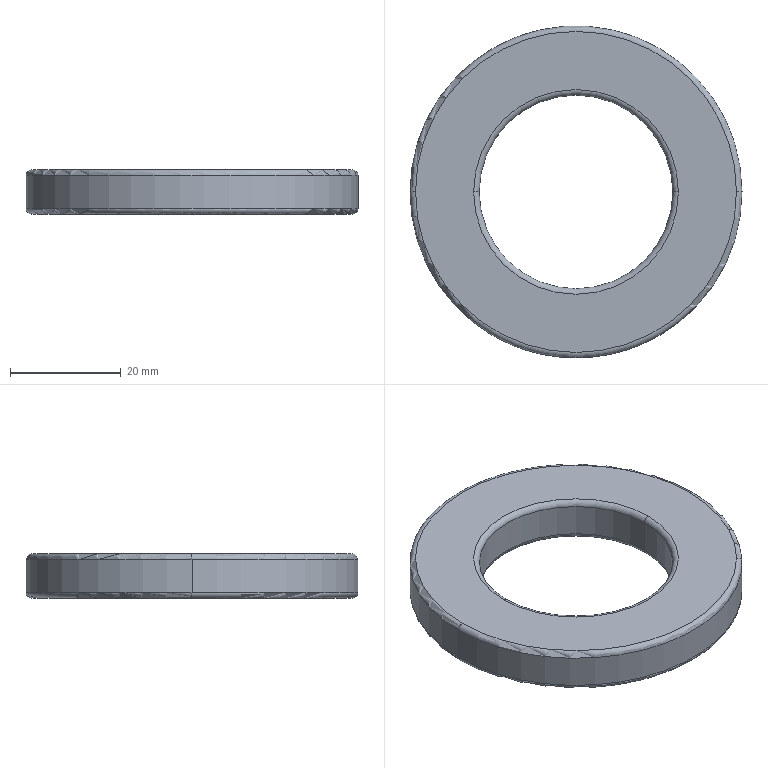Part | SolidWorks | features Extrusion 1, Fillet 1 | 1 solid | 14 faces | box 60 x 60 x 8 mm | volume 14794 mm3 | torus 8 | cylinder 4 | plane 2 | commonest cylinder face diameters 35 x2 60 x2
STEP:
#1=CARTESIAN_POINT('',(-30.,0.,7.));
#2=VERTEX_POINT('',#1);
#3=CARTESIAN_POINT('',(30.,0.,7.));
#4=VERTEX_POINT('',#3);
#5=CARTESIAN_POINT('',(0.,0.,7.));
#6=DIRECTION('',(0.,0.,-1.));
#7=DIRECTION('',(1.,0.,0.));
#8=AXIS2_PLACEMENT_3D('',#5,#6,#7);
#9=CIRCLE('',#8,30.);
#10=EDGE_CURVE('',#2,#4,#9,.T.);
#11=ORIENTED_EDGE('',*,*,#10,.F.);
#12=CARTESIAN_POINT('',(-29.,0.,8.));
#13=VERTEX_POINT('',#12);
#14=CARTESIAN_POINT('',(-29.,0.,7.));
#15=DIRECTION('',(0.,1.,0.));
#16=DIRECTION('',(-1.,0.,0.));
#17=AXIS2_PLACEMENT_3D('',#14,#15,#16);
#18=CIRCLE('',#17,1.);
#19=EDGE_CURVE('',#2,#13,#18,.T.);
#20=ORIENTED_EDGE('',*,*,#19,.T.);
#21=CARTESIAN_POINT('',(29.,0.,8.));
#22=VERTEX_POINT('',#21);
#23=CARTESIAN_POINT('',(0.,0.,8.));
#24=DIRECTION('',(0.,0.,1.));
#25=DIRECTION('',(1.,0.,0.));
#26=AXIS2_PLACEMENT_3D('',#23,#24,#25);
#27=CIRCLE('',#26,29.);
#28=EDGE_CURVE('',#22,#13,#27,.T.);
#29=ORIENTED_EDGE('',*,*,#28,.F.);
#30=CARTESIAN_POINT('',(29.,0.,7.));
#31=DIRECTION('',(0.,-1.,0.));
#32=DIRECTION('',(0.,0.,-1.));
#33=AXIS2_PLACEMENT_3D('',#30,#31,#32);
#34=CIRCLE('',#33,1.);
#35=EDGE_CURVE('',#4,#22,#34,.T.);
#36=ORIENTED_EDGE('',*,*,#35,.F.);
#37=EDGE_LOOP('',(#11,#20,#29,#36));
#38=FACE_OUTER_BOUND('',#37,.T.);
#39=CARTESIAN_POINT('',(0.,0.,7.));
#40=DIRECTION('',(0.,0.,1.));
#41=DIRECTION('',(1.,0.,0.));
#42=AXIS2_PLACEMENT_3D('',#39,#40,#41);
#43=TOROIDAL_SURFACE('',#42,29.,1.);
#44=ADVANCED_FACE('',(#38),#43,.T.);
#45=CARTESIAN_POINT('',(-29.,0.,0.));
#46=VERTEX_POINT('',#45);
#47=CARTESIAN_POINT('',(29.,0.,0.));
#48=VERTEX_POINT('',#47);
#49=CARTESIAN_POINT('',(0.,0.,0.));
#50=DIRECTION('',(0.,0.,-1.));
#51=DIRECTION('',(1.,0.,0.));
#52=AXIS2_PLACEMENT_3D('',#49,#50,#51);
#53=CIRCLE('',#52,29.);
#54=EDGE_CURVE('',#46,#48,#53,.T.);
#55=ORIENTED_EDGE('',*,*,#54,.F.);
#56=CARTESIAN_POINT('',(-30.,0.,1.));
#57=VERTEX_POINT('',#56);
#58=CARTESIAN_POINT('',(-29.,0.,1.));
#59=DIRECTION('',(0.,1.,0.));
#60=DIRECTION('',(-1.,0.,0.));
#61=AXIS2_PLACEMENT_3D('',#58,#59,#60);
#62=CIRCLE('',#61,1.);
#63=EDGE_CURVE('',#46,#57,#62,.T.);
#64=ORIENTED_EDGE('',*,*,#63,.T.);
#65=CARTESIAN_POINT('',(30.,0.,1.));
#66=VERTEX_POINT('',#65);
#67=CARTESIAN_POINT('',(0.,0.,1.));
#68=DIRECTION('',(0.,0.,1.));
#69=DIRECTION('',(1.,0.,0.));
#70=AXIS2_PLACEMENT_3D('',#67,#68,#69);
#71=CIRCLE('',#70,30.);
#72=EDGE_CURVE('',#66,#57,#71,.T.);
#73=ORIENTED_EDGE('',*,*,#72,.F.);
#74=CARTESIAN_POINT('',(29.,0.,1.));
#75=DIRECTION('',(0.,-1.,0.));
#76=DIRECTION('',(0.,0.,-1.));
#77=AXIS2_PLACEMENT_3D('',#74,#75,#76);
#78=CIRCLE('',#77,1.);
#79=EDGE_CURVE('',#48,#66,#78,.T.);
#80=ORIENTED_EDGE('',*,*,#79,.F.);
#81=EDGE_LOOP('',(#55,#64,#73,#80));
#82=FACE_OUTER_BOUND('',#81,.T.);
#83=CARTESIAN_POINT('',(0.,0.,1.));
#84=DIRECTION('',(0.,0.,1.));
#85=DIRECTION('',(1.,0.,0.));
#86=AXIS2_PLACEMENT_3D('',#83,#84,#85);
#87=TOROIDAL_SURFACE('',#86,29.,1.);
#88=ADVANCED_FACE('',(#82),#87,.T.);
#89=CARTESIAN_POINT('',(-18.5,0.,8.));
#90=VERTEX_POINT('',#89);
#91=CARTESIAN_POINT('',(18.5,0.,8.));
#92=VERTEX_POINT('',#91);
#93=CARTESIAN_POINT('',(0.,0.,8.));
#94=DIRECTION('',(0.,0.,-1.));
#95=DIRECTION('',(1.,0.,0.));
#96=AXIS2_PLACEMENT_3D('',#93,#94,#95);
#97=CIRCLE('',#96,18.5);
#98=EDGE_CURVE('',#90,#92,#97,.T.);
#99=ORIENTED_EDGE('',*,*,#98,.F.);
#100=CARTESIAN_POINT('',(-17.5,0.,7.));
#101=VERTEX_POINT('',#100);
#102=CARTESIAN_POINT('',(-18.5,0.,7.));
#103=DIRECTION('',(0.,1.,0.));
#104=DIRECTION('',(-1.,0.,0.));
#105=AXIS2_PLACEMENT_3D('',#102,#103,#104);
#106=CIRCLE('',#105,1.);
#107=EDGE_CURVE('',#90,#101,#106,.T.);
#108=ORIENTED_EDGE('',*,*,#107,.T.);
#109=CARTESIAN_POINT('',(17.5,0.,7.));
#110=VERTEX_POINT('',#109);
#111=CARTESIAN_POINT('',(0.,0.,7.));
#112=DIRECTION('',(0.,0.,1.));
#113=DIRECTION('',(1.,0.,0.));
#114=AXIS2_PLACEMENT_3D('',#111,#112,#113);
#115=CIRCLE('',#114,17.5);
#116=EDGE_CURVE('',#110,#101,#115,.T.);
#117=ORIENTED_EDGE('',*,*,#116,.F.);
#118=CARTESIAN_POINT('',(18.5,0.,7.));
#119=DIRECTION('',(0.,-1.,0.));
#120=DIRECTION('',(0.,0.,-1.));
#121=AXIS2_PLACEMENT_3D('',#118,#119,#120);
#122=CIRCLE('',#121,1.);
#123=EDGE_CURVE('',#92,#110,#122,.T.);
#124=ORIENTED_EDGE('',*,*,#123,.F.);
#125=EDGE_LOOP('',(#99,#108,#117,#124));
#126=FACE_OUTER_BOUND('',#125,.T.);
#127=CARTESIAN_POINT('',(0.,0.,7.));
#128=DIRECTION('',(0.,0.,1.));
#129=DIRECTION('',(1.,0.,0.));
#130=AXIS2_PLACEMENT_3D('',#127,#128,#129);
#131=TOROIDAL_SURFACE('',#130,18.5,1.);
#132=ADVANCED_FACE('',(#126),#131,.T.);
#133=CARTESIAN_POINT('',(-17.5,0.,1.));
#134=VERTEX_POINT('',#133);
#135=CARTESIAN_POINT('',(17.5,0.,1.));
#136=VERTEX_POINT('',#135);
#137=CARTESIAN_POINT('',(0.,0.,1.));
#138=DIRECTION('',(0.,0.,-1.));
#139=DIRECTION('',(1.,0.,0.));
#140=AXIS2_PLACEMENT_3D('',#137,#138,#139);
#141=CIRCLE('',#140,17.5);
#142=EDGE_CURVE('',#134,#136,#141,.T.);
#143=ORIENTED_EDGE('',*,*,#142,.F.);
#144=CARTESIAN_POINT('',(-18.5,0.,0.));
#145=VERTEX_POINT('',#144);
#146=CARTESIAN_POINT('',(-18.5,0.,1.));
#147=DIRECTION('',(0.,1.,0.));
#148=DIRECTION('',(-1.,0.,0.));
#149=AXIS2_PLACEMENT_3D('',#146,#147,#148);
#150=CIRCLE('',#149,1.);
#151=EDGE_CURVE('',#134,#145,#150,.T.);
#152=ORIENTED_EDGE('',*,*,#151,.T.);
#153=CARTESIAN_POINT('',(18.5,0.,0.));
#154=VERTEX_POINT('',#153);
#155=CARTESIAN_POINT('',(0.,0.,0.));
#156=DIRECTION('',(0.,0.,1.));
#157=DIRECTION('',(1.,0.,0.));
#158=AXIS2_PLACEMENT_3D('',#155,#156,#157);
#159=CIRCLE('',#158,18.5);
#160=EDGE_CURVE('',#154,#145,#159,.T.);
#161=ORIENTED_EDGE('',*,*,#160,.F.);
#162=CARTESIAN_POINT('',(18.5,0.,1.));
#163=DIRECTION('',(0.,-1.,0.));
#164=DIRECTION('',(0.,0.,-1.));
#165=AXIS2_PLACEMENT_3D('',#162,#163,#164);
#166=CIRCLE('',#165,1.);
#167=EDGE_CURVE('',#136,#154,#166,.T.);
#168=ORIENTED_EDGE('',*,*,#167,.F.);
#169=EDGE_LOOP('',(#143,#152,#161,#168));
#170=FACE_OUTER_BOUND('',#169,.T.);
#171=CARTESIAN_POINT('',(0.,0.,1.));
#172=DIRECTION('',(0.,0.,1.));
#173=DIRECTION('',(1.,0.,0.));
#174=AXIS2_PLACEMENT_3D('',#171,#172,#173);
#175=TOROIDAL_SURFACE('',#174,18.5,1.);
#176=ADVANCED_FACE('',(#170),#175,.T.);
#177=CARTESIAN_POINT('',(0.,0.,7.));
#178=DIRECTION('',(0.,0.,1.));
#179=DIRECTION('',(1.,0.,0.));
#180=AXIS2_PLACEMENT_3D('',#177,#178,#179);
#181=CIRCLE('',#180,17.5);
#182=EDGE_CURVE('',#101,#110,#181,.T.);
#183=ORIENTED_EDGE('',*,*,#182,.T.);
#184=CARTESIAN_POINT('',(17.5,0.,8.));
#185=DIRECTION('',(0.,0.,-1.));
#186=VECTOR('',#185,1000.);
#187=LINE('',#184,#186);
#188=EDGE_CURVE('',#110,#136,#187,.T.);
#189=ORIENTED_EDGE('',*,*,#188,.T.);
#190=CARTESIAN_POINT('',(0.,0.,1.));
#191=DIRECTION('',(0.,0.,-1.));
#192=DIRECTION('',(1.,0.,0.));
#193=AXIS2_PLACEMENT_3D('',#190,#191,#192);
#194=CIRCLE('',#193,17.5);
#195=EDGE_CURVE('',#136,#134,#194,.T.);
#196=ORIENTED_EDGE('',*,*,#195,.T.);
#197=CARTESIAN_POINT('',(-17.5,0.,8.));
#198=DIRECTION('',(0.,0.,-1.));
#199=VECTOR('',#198,1000.);
#200=LINE('',#197,#199);
#201=EDGE_CURVE('',#101,#134,#200,.T.);
#202=ORIENTED_EDGE('',*,*,#201,.F.);
#203=EDGE_LOOP('',(#183,#189,#196,#202));
#204=FACE_OUTER_BOUND('',#203,.T.);
#205=CARTESIAN_POINT('',(0.,0.,8.));
#206=DIRECTION('',(0.,0.,-1.));
#207=DIRECTION('',(-1.,0.,0.));
#208=AXIS2_PLACEMENT_3D('',#205,#206,#207);
#209=CYLINDRICAL_SURFACE('',#208,17.5);
#210=ADVANCED_FACE('',(#204),#209,.F.);
#211=ORIENTED_EDGE('',*,*,#10,.T.);
#212=CARTESIAN_POINT('',(30.,0.,8.));
#213=DIRECTION('',(0.,0.,-1.));
#214=VECTOR('',#213,1000.);
#215=LINE('',#212,#214);
#216=EDGE_CURVE('',#4,#66,#215,.T.);
#217=ORIENTED_EDGE('',*,*,#216,.T.);
#218=ORIENTED_EDGE('',*,*,#72,.T.);
#219=CARTESIAN_POINT('',(-30.,0.,8.));
#220=DIRECTION('',(0.,0.,-1.));
#221=VECTOR('',#220,1000.);
#222=LINE('',#219,#221);
#223=EDGE_CURVE('',#2,#57,#222,.T.);
#224=ORIENTED_EDGE('',*,*,#223,.F.);
#225=EDGE_LOOP('',(#211,#217,#218,#224));
#226=FACE_OUTER_BOUND('',#225,.T.);
#227=CARTESIAN_POINT('',(0.,0.,8.));
#228=DIRECTION('',(0.,0.,-1.));
#229=DIRECTION('',(-1.,0.,0.));
#230=AXIS2_PLACEMENT_3D('',#227,#228,#229);
#231=CYLINDRICAL_SURFACE('',#230,30.);
#232=ADVANCED_FACE('',(#226),#231,.T.);
#233=CARTESIAN_POINT('',(0.,0.,8.));
#234=DIRECTION('',(0.,0.,-1.));
#235=DIRECTION('',(1.,0.,0.));
#236=AXIS2_PLACEMENT_3D('',#233,#234,#235);
#237=CIRCLE('',#236,18.5);
#238=EDGE_CURVE('',#92,#90,#237,.T.);
#239=ORIENTED_EDGE('',*,*,#238,.T.);
#240=ORIENTED_EDGE('',*,*,#98,.T.);
#241=EDGE_LOOP('',(#239,#240));
#242=FACE_BOUND('',#241,.T.);
#243=ORIENTED_EDGE('',*,*,#28,.T.);
#244=CARTESIAN_POINT('',(0.,0.,8.));
#245=DIRECTION('',(0.,0.,1.));
#246=DIRECTION('',(1.,0.,0.));
#247=AXIS2_PLACEMENT_3D('',#244,#245,#246);
#248=CIRCLE('',#247,29.);
#249=EDGE_CURVE('',#13,#22,#248,.T.);
#250=ORIENTED_EDGE('',*,*,#249,.T.);
#251=EDGE_LOOP('',(#243,#250));
#252=FACE_OUTER_BOUND('',#251,.T.);
#253=CARTESIAN_POINT('',(0.,0.,8.));
#254=DIRECTION('',(0.,0.,1.));
#255=DIRECTION('',(1.,0.,0.));
#256=AXIS2_PLACEMENT_3D('',#253,#254,#255);
#257=PLANE('',#256);
#258=ADVANCED_FACE('',(#242,#252),#257,.T.);
#259=ORIENTED_EDGE('',*,*,#160,.T.);
#260=CARTESIAN_POINT('',(0.,0.,0.));
#261=DIRECTION('',(0.,0.,1.));
#262=DIRECTION('',(1.,0.,0.));
#263=AXIS2_PLACEMENT_3D('',#260,#261,#262);
#264=CIRCLE('',#263,18.5);
#265=EDGE_CURVE('',#145,#154,#264,.T.);
#266=ORIENTED_EDGE('',*,*,#265,.T.);
#267=EDGE_LOOP('',(#259,#266));
#268=FACE_BOUND('',#267,.T.);
#269=CARTESIAN_POINT('',(0.,0.,0.));
#270=DIRECTION('',(0.,0.,-1.));
#271=DIRECTION('',(1.,0.,0.));
#272=AXIS2_PLACEMENT_3D('',#269,#270,#271);
#273=CIRCLE('',#272,29.);
#274=EDGE_CURVE('',#48,#46,#273,.T.);
#275=ORIENTED_EDGE('',*,*,#274,.T.);
#276=ORIENTED_EDGE('',*,*,#54,.T.);
#277=EDGE_LOOP('',(#275,#276));
#278=FACE_OUTER_BOUND('',#277,.T.);
#279=CARTESIAN_POINT('',(0.,0.,0.));
#280=DIRECTION('',(0.,0.,1.));
#281=DIRECTION('',(1.,0.,0.));
#282=AXIS2_PLACEMENT_3D('',#279,#280,#281);
#283=PLANE('',#282);
#284=ADVANCED_FACE('',(#268,#278),#283,.F.);
#285=ORIENTED_EDGE('',*,*,#216,.F.);
#286=CARTESIAN_POINT('',(0.,0.,7.));
#287=DIRECTION('',(0.,0.,-1.));
#288=DIRECTION('',(1.,0.,0.));
#289=AXIS2_PLACEMENT_3D('',#286,#287,#288);
#290=CIRCLE('',#289,30.);
#291=EDGE_CURVE('',#4,#2,#290,.T.);
#292=ORIENTED_EDGE('',*,*,#291,.T.);
#293=ORIENTED_EDGE('',*,*,#223,.T.);
#294=CARTESIAN_POINT('',(0.,0.,1.));
#295=DIRECTION('',(0.,0.,1.));
#296=DIRECTION('',(1.,0.,0.));
#297=AXIS2_PLACEMENT_3D('',#294,#295,#296);
#298=CIRCLE('',#297,30.);
#299=EDGE_CURVE('',#57,#66,#298,.T.);
#300=ORIENTED_EDGE('',*,*,#299,.T.);
#301=EDGE_LOOP('',(#285,#292,#293,#300));
#302=FACE_OUTER_BOUND('',#301,.T.);
#303=CARTESIAN_POINT('',(0.,0.,8.));
#304=DIRECTION('',(0.,0.,-1.));
#305=DIRECTION('',(-1.,0.,0.));
#306=AXIS2_PLACEMENT_3D('',#303,#304,#305);
#307=CYLINDRICAL_SURFACE('',#306,30.);
#308=ADVANCED_FACE('',(#302),#307,.T.);
#309=ORIENTED_EDGE('',*,*,#188,.F.);
#310=ORIENTED_EDGE('',*,*,#116,.T.);
#311=ORIENTED_EDGE('',*,*,#201,.T.);
#312=ORIENTED_EDGE('',*,*,#142,.T.);
#313=EDGE_LOOP('',(#309,#310,#311,#312));
#314=FACE_OUTER_BOUND('',#313,.T.);
#315=CARTESIAN_POINT('',(0.,0.,8.));
#316=DIRECTION('',(0.,0.,-1.));
#317=DIRECTION('',(-1.,0.,0.));
#318=AXIS2_PLACEMENT_3D('',#315,#316,#317);
#319=CYLINDRICAL_SURFACE('',#318,17.5);
#320=ADVANCED_FACE('',(#314),#319,.F.);
#321=ORIENTED_EDGE('',*,*,#151,.F.);
#322=ORIENTED_EDGE('',*,*,#195,.F.);
#323=ORIENTED_EDGE('',*,*,#167,.T.);
#324=ORIENTED_EDGE('',*,*,#265,.F.);
#325=EDGE_LOOP('',(#321,#322,#323,#324));
#326=FACE_OUTER_BOUND('',#325,.T.);
#327=CARTESIAN_POINT('',(0.,0.,1.));
#328=DIRECTION('',(0.,0.,1.));
#329=DIRECTION('',(1.,0.,0.));
#330=AXIS2_PLACEMENT_3D('',#327,#328,#329);
#331=TOROIDAL_SURFACE('',#330,18.5,1.);
#332=ADVANCED_FACE('',(#326),#331,.T.);
#333=ORIENTED_EDGE('',*,*,#107,.F.);
#334=ORIENTED_EDGE('',*,*,#238,.F.);
#335=ORIENTED_EDGE('',*,*,#123,.T.);
#336=ORIENTED_EDGE('',*,*,#182,.F.);
#337=EDGE_LOOP('',(#333,#334,#335,#336));
#338=FACE_OUTER_BOUND('',#337,.T.);
#339=CARTESIAN_POINT('',(0.,0.,7.));
#340=DIRECTION('',(0.,0.,1.));
#341=DIRECTION('',(1.,0.,0.));
#342=AXIS2_PLACEMENT_3D('',#339,#340,#341);
#343=TOROIDAL_SURFACE('',#342,18.5,1.);
#344=ADVANCED_FACE('',(#338),#343,.T.);
#345=ORIENTED_EDGE('',*,*,#63,.F.);
#346=ORIENTED_EDGE('',*,*,#274,.F.);
#347=ORIENTED_EDGE('',*,*,#79,.T.);
#348=ORIENTED_EDGE('',*,*,#299,.F.);
#349=EDGE_LOOP('',(#345,#346,#347,#348));
#350=FACE_OUTER_BOUND('',#349,.T.);
#351=CARTESIAN_POINT('',(0.,0.,1.));
#352=DIRECTION('',(0.,0.,1.));
#353=DIRECTION('',(1.,0.,0.));
#354=AXIS2_PLACEMENT_3D('',#351,#352,#353);
#355=TOROIDAL_SURFACE('',#354,29.,1.);
#356=ADVANCED_FACE('',(#350),#355,.T.);
#357=ORIENTED_EDGE('',*,*,#19,.F.);
#358=ORIENTED_EDGE('',*,*,#291,.F.);
#359=ORIENTED_EDGE('',*,*,#35,.T.);
#360=ORIENTED_EDGE('',*,*,#249,.F.);
#361=EDGE_LOOP('',(#357,#358,#359,#360));
#362=FACE_OUTER_BOUND('',#361,.T.);
#363=CARTESIAN_POINT('',(0.,0.,7.));
#364=DIRECTION('',(0.,0.,1.));
#365=DIRECTION('',(1.,0.,0.));
#366=AXIS2_PLACEMENT_3D('',#363,#364,#365);
#367=TOROIDAL_SURFACE('',#366,29.,1.);
#368=ADVANCED_FACE('',(#362),#367,.T.);
#369=CLOSED_SHELL('',(#44,#88,#132,#176,#210,#232,#258,#284,#308,#320,#332,#344,#356,#368));
#370=MANIFOLD_SOLID_BREP('',#369);
#371=CARTESIAN_POINT('',(0.,0.,0.));
#372=DIRECTION('',(0.,0.,1.));
#373=DIRECTION('',(1.,0.,0.));
#374=AXIS2_PLACEMENT_3D('',#371,#372,#373);
#375=(LENGTH_UNIT()NAMED_UNIT(*)SI_UNIT(.MILLI.,.METRE.));
#376=UNCERTAINTY_MEASURE_WITH_UNIT(LENGTH_MEASURE(0.00001),#375,'','');
#377=(NAMED_UNIT(*)PLANE_ANGLE_UNIT()SI_UNIT($,.RADIAN.));
#378=(NAMED_UNIT(*)SI_UNIT($,.STERADIAN.)SOLID_ANGLE_UNIT());
#379=(GEOMETRIC_REPRESENTATION_CONTEXT(3)GLOBAL_UNCERTAINTY_ASSIGNED_CONTEXT((#376))GLOBAL_UNIT_ASSIGNED_CONTEXT((#375,#377,#378))REPRESENTATION_CONTEXT('',''));
#380=ADVANCED_BREP_SHAPE_REPRESENTATION('',(#370,#374),#379);